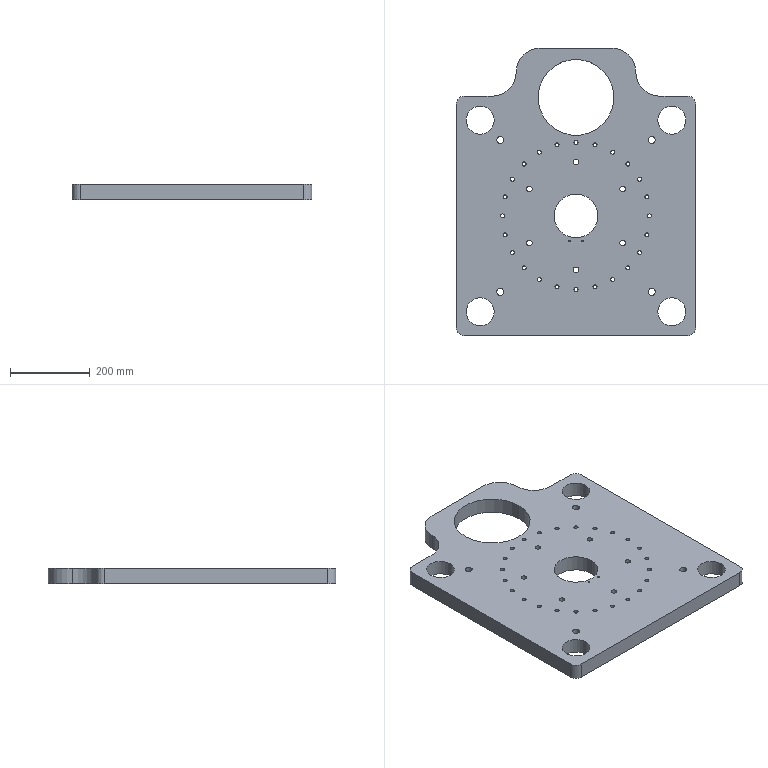Part | SolidWorks | features Extrusion 1, HoleWzd 1, ICE 1, LPattern 1 | 1 solid | 160 faces | box 600 x 720 x 40 mm | volume 13513798 mm3 | cylinder 124 | cone 24 | plane 12 | commonest cylinder face diameters 10.106 x48 3.2 x24 13.835 x12 17.294 x8 70 x8 98 x8